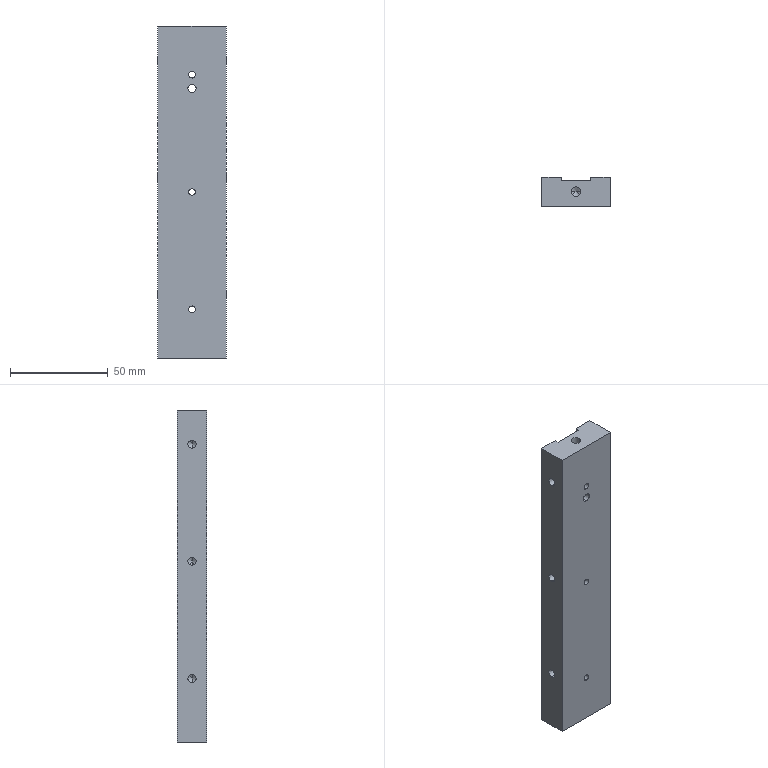Part | STEP file | A14-022 | 1 solid | 50 faces | box 35 x 15 x 170 mm | volume 81962 mm3 | cylinder 24 | cone 16 | plane 10 | commonest cylinder face diameters 4.2 x14 3.3 x6 5 x4